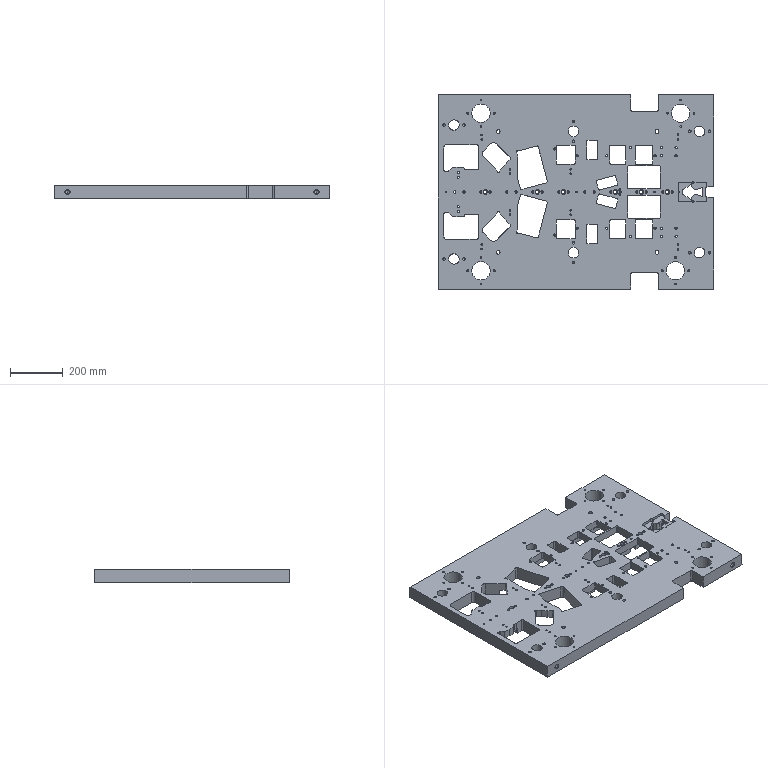Part | NX | features solid 2 | 1 solid | 602 faces | box 1047 x 740 x 50 mm | volume 27945146 mm3 | cylinder 300 | plane 213 | cone 74 | spline 15 | commonest cylinder face diameters 8 x56 10 x44 6.806 x42 6.805 x20 8.5 x20 8.506 x18